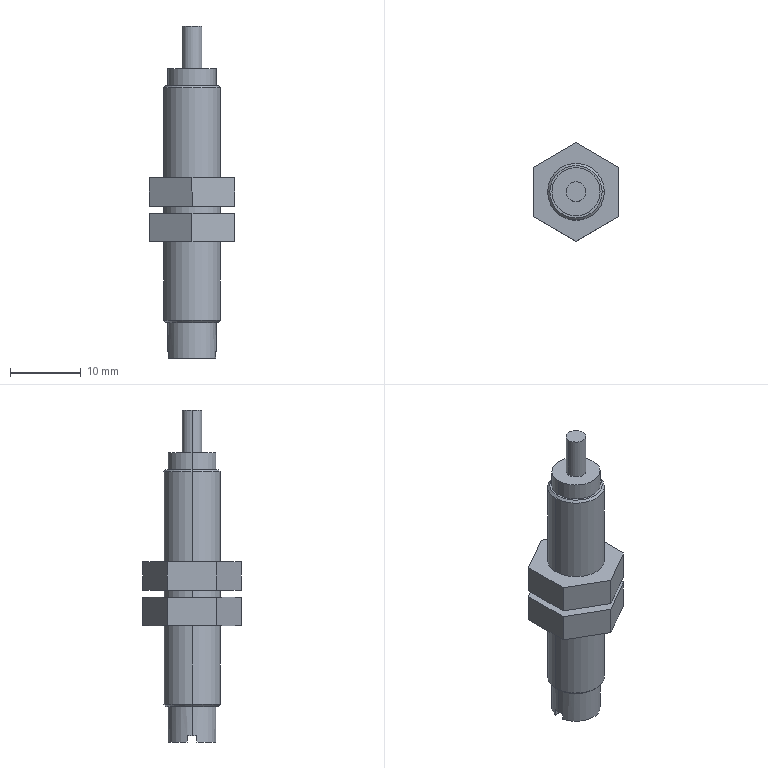Part | SolidWorks | features BaseBody 1 | 1 solid | 41 faces | box 12 x 13.856 x 46.8 mm | volume 2569 mm3 | plane 25 | cylinder 12 | cone 4 | commonest cylinder face diameters 8 x6 6.8 x4 2.8 x2
STEP:
#1=CARTESIAN_POINT('',(1.4,0.,0.));
#2=VERTEX_POINT('',#1);
#3=CARTESIAN_POINT('',(-1.4,0.,0.));
#4=VERTEX_POINT('',#3);
#5=CARTESIAN_POINT('',(0.,0.,0.));
#6=DIRECTION('',(0.,0.,1.));
#7=DIRECTION('',(1.,0.,0.));
#8=AXIS2_PLACEMENT_3D('',#5,#6,#7);
#9=CIRCLE('',#8,1.4);
#10=EDGE_CURVE('',#2,#4,#9,.T.);
#11=ORIENTED_EDGE('',*,*,#10,.T.);
#12=CARTESIAN_POINT('',(-1.4,0.,6.));
#13=VERTEX_POINT('',#12);
#14=CARTESIAN_POINT('',(-1.4,0.,6.));
#15=DIRECTION('',(0.,0.,1.));
#16=VECTOR('',#15,1000.);
#17=LINE('',#14,#16);
#18=EDGE_CURVE('',#4,#13,#17,.T.);
#19=ORIENTED_EDGE('',*,*,#18,.T.);
#20=CARTESIAN_POINT('',(1.4,0.,6.));
#21=VERTEX_POINT('',#20);
#22=CARTESIAN_POINT('',(0.,0.,6.));
#23=DIRECTION('',(0.,0.,-1.));
#24=DIRECTION('',(1.,0.,0.));
#25=AXIS2_PLACEMENT_3D('',#22,#23,#24);
#26=CIRCLE('',#25,1.4);
#27=EDGE_CURVE('',#13,#21,#26,.T.);
#28=ORIENTED_EDGE('',*,*,#27,.T.);
#29=CARTESIAN_POINT('',(1.4,0.,6.));
#30=DIRECTION('',(0.,0.,1.));
#31=VECTOR('',#30,1000.);
#32=LINE('',#29,#31);
#33=EDGE_CURVE('',#2,#21,#32,.T.);
#34=ORIENTED_EDGE('',*,*,#33,.F.);
#35=EDGE_LOOP('',(#11,#19,#28,#34));
#36=FACE_OUTER_BOUND('',#35,.T.);
#37=CARTESIAN_POINT('',(0.,0.,6.));
#38=DIRECTION('',(0.,0.,1.));
#39=DIRECTION('',(1.,0.,0.));
#40=AXIS2_PLACEMENT_3D('',#37,#38,#39);
#41=CYLINDRICAL_SURFACE('',#40,1.4);
#42=ADVANCED_FACE('',(#36),#41,.T.);
#43=CARTESIAN_POINT('',(3.4,0.,-2.4));
#44=VERTEX_POINT('',#43);
#45=CARTESIAN_POINT('',(-3.4,0.,-2.4));
#46=VERTEX_POINT('',#45);
#47=CARTESIAN_POINT('',(0.,0.,-2.4));
#48=DIRECTION('',(0.,0.,1.));
#49=DIRECTION('',(1.,0.,0.));
#50=AXIS2_PLACEMENT_3D('',#47,#48,#49);
#51=CIRCLE('',#50,3.4);
#52=EDGE_CURVE('',#44,#46,#51,.T.);
#53=ORIENTED_EDGE('',*,*,#52,.T.);
#54=CARTESIAN_POINT('',(-3.4,0.,0.));
#55=VERTEX_POINT('',#54);
#56=CARTESIAN_POINT('',(-3.4,0.,0.));
#57=DIRECTION('',(0.,0.,1.));
#58=VECTOR('',#57,1000.);
#59=LINE('',#56,#58);
#60=EDGE_CURVE('',#46,#55,#59,.T.);
#61=ORIENTED_EDGE('',*,*,#60,.T.);
#62=CARTESIAN_POINT('',(3.4,0.,0.));
#63=VERTEX_POINT('',#62);
#64=CARTESIAN_POINT('',(0.,0.,0.));
#65=DIRECTION('',(0.,0.,1.));
#66=DIRECTION('',(1.,0.,0.));
#67=AXIS2_PLACEMENT_3D('',#64,#65,#66);
#68=CIRCLE('',#67,3.4);
#69=EDGE_CURVE('',#63,#55,#68,.T.);
#70=ORIENTED_EDGE('',*,*,#69,.F.);
#71=CARTESIAN_POINT('',(3.4,0.,0.));
#72=DIRECTION('',(0.,0.,1.));
#73=VECTOR('',#72,1000.);
#74=LINE('',#71,#73);
#75=EDGE_CURVE('',#44,#63,#74,.T.);
#76=ORIENTED_EDGE('',*,*,#75,.F.);
#77=EDGE_LOOP('',(#53,#61,#70,#76));
#78=FACE_OUTER_BOUND('',#77,.T.);
#79=CARTESIAN_POINT('',(0.,0.,0.));
#80=DIRECTION('',(0.,0.,1.));
#81=DIRECTION('',(1.,0.,0.));
#82=AXIS2_PLACEMENT_3D('',#79,#80,#81);
#83=CYLINDRICAL_SURFACE('',#82,3.4);
#84=ADVANCED_FACE('',(#78),#83,.T.);
#85=CARTESIAN_POINT('',(3.694,0.,-2.4));
#86=VERTEX_POINT('',#85);
#87=CARTESIAN_POINT('',(-3.694,0.,-2.4));
#88=VERTEX_POINT('',#87);
#89=CARTESIAN_POINT('',(0.,0.,-2.4));
#90=DIRECTION('',(0.,0.,1.));
#91=DIRECTION('',(-1.,0.,0.));
#92=AXIS2_PLACEMENT_3D('',#89,#90,#91);
#93=CIRCLE('',#92,3.694);
#94=EDGE_CURVE('',#86,#88,#93,.T.);
#95=ORIENTED_EDGE('',*,*,#94,.F.);
#96=CARTESIAN_POINT('',(4.,0.,-2.707));
#97=VERTEX_POINT('',#96);
#98=CARTESIAN_POINT('',(3.694,0.,-2.4));
#99=DIRECTION('',(0.7071,0.,-0.7071));
#100=VECTOR('',#99,1000.);
#101=LINE('',#98,#100);
#102=EDGE_CURVE('',#86,#97,#101,.T.);
#103=ORIENTED_EDGE('',*,*,#102,.T.);
#104=CARTESIAN_POINT('',(-4.,0.,-2.707));
#105=VERTEX_POINT('',#104);
#106=CARTESIAN_POINT('',(0.,0.,-2.707));
#107=DIRECTION('',(0.,0.,1.));
#108=DIRECTION('',(0.,1.,0.));
#109=AXIS2_PLACEMENT_3D('',#106,#107,#108);
#110=CIRCLE('',#109,4.);
#111=EDGE_CURVE('',#97,#105,#110,.T.);
#112=ORIENTED_EDGE('',*,*,#111,.T.);
#113=CARTESIAN_POINT('',(-3.694,0.,-2.4));
#114=DIRECTION('',(-0.7071,0.,-0.7071));
#115=VECTOR('',#114,1000.);
#116=LINE('',#113,#115);
#117=EDGE_CURVE('',#88,#105,#116,.T.);
#118=ORIENTED_EDGE('',*,*,#117,.F.);
#119=EDGE_LOOP('',(#95,#103,#112,#118));
#120=FACE_OUTER_BOUND('',#119,.T.);
#121=CARTESIAN_POINT('',(0.,0.,-2.4));
#122=DIRECTION('',(0.,0.,-1.));
#123=DIRECTION('',(-1.,0.,0.));
#124=AXIS2_PLACEMENT_3D('',#121,#122,#123);
#125=CONICAL_SURFACE('',#124,3.694,0.7854);
#126=ADVANCED_FACE('',(#120),#125,.T.);
#127=CARTESIAN_POINT('',(4.,0.,-15.4));
#128=VERTEX_POINT('',#127);
#129=CARTESIAN_POINT('',(-4.,0.,-15.4));
#130=VERTEX_POINT('',#129);
#131=CARTESIAN_POINT('',(0.,0.,-15.4));
#132=DIRECTION('',(0.,0.,1.));
#133=DIRECTION('',(1.,0.,0.));
#134=AXIS2_PLACEMENT_3D('',#131,#132,#133);
#135=CIRCLE('',#134,4.);
#136=EDGE_CURVE('',#128,#130,#135,.T.);
#137=ORIENTED_EDGE('',*,*,#136,.T.);
#138=CARTESIAN_POINT('',(-4.,0.,-2.707));
#139=DIRECTION('',(0.,0.,1.));
#140=VECTOR('',#139,1000.);
#141=LINE('',#138,#140);
#142=EDGE_CURVE('',#130,#105,#141,.T.);
#143=ORIENTED_EDGE('',*,*,#142,.T.);
#144=ORIENTED_EDGE('',*,*,#111,.F.);
#145=CARTESIAN_POINT('',(4.,0.,-2.707));
#146=DIRECTION('',(0.,0.,1.));
#147=VECTOR('',#146,1000.);
#148=LINE('',#145,#147);
#149=EDGE_CURVE('',#128,#97,#148,.T.);
#150=ORIENTED_EDGE('',*,*,#149,.F.);
#151=EDGE_LOOP('',(#137,#143,#144,#150));
#152=FACE_OUTER_BOUND('',#151,.T.);
#153=CARTESIAN_POINT('',(0.,0.,-2.707));
#154=DIRECTION('',(0.,0.,1.));
#155=DIRECTION('',(1.,0.,0.));
#156=AXIS2_PLACEMENT_3D('',#153,#154,#155);
#157=CYLINDRICAL_SURFACE('',#156,4.);
#158=ADVANCED_FACE('',(#152),#157,.T.);
#159=CARTESIAN_POINT('',(4.,0.,-20.4));
#160=VERTEX_POINT('',#159);
#161=CARTESIAN_POINT('',(-4.,0.,-20.4));
#162=VERTEX_POINT('',#161);
#163=CARTESIAN_POINT('',(0.,0.,-20.4));
#164=DIRECTION('',(0.,0.,1.));
#165=DIRECTION('',(1.,0.,0.));
#166=AXIS2_PLACEMENT_3D('',#163,#164,#165);
#167=CIRCLE('',#166,4.);
#168=EDGE_CURVE('',#160,#162,#167,.T.);
#169=ORIENTED_EDGE('',*,*,#168,.T.);
#170=CARTESIAN_POINT('',(-4.,0.,-19.4));
#171=VERTEX_POINT('',#170);
#172=CARTESIAN_POINT('',(-4.,0.,-19.4));
#173=DIRECTION('',(0.,0.,1.));
#174=VECTOR('',#173,1000.);
#175=LINE('',#172,#174);
#176=EDGE_CURVE('',#162,#171,#175,.T.);
#177=ORIENTED_EDGE('',*,*,#176,.T.);
#178=CARTESIAN_POINT('',(4.,0.,-19.4));
#179=VERTEX_POINT('',#178);
#180=CARTESIAN_POINT('',(0.,0.,-19.4));
#181=DIRECTION('',(0.,0.,1.));
#182=DIRECTION('',(1.,0.,0.));
#183=AXIS2_PLACEMENT_3D('',#180,#181,#182);
#184=CIRCLE('',#183,4.);
#185=EDGE_CURVE('',#179,#171,#184,.T.);
#186=ORIENTED_EDGE('',*,*,#185,.F.);
#187=CARTESIAN_POINT('',(4.,0.,-19.4));
#188=DIRECTION('',(0.,0.,1.));
#189=VECTOR('',#188,1000.);
#190=LINE('',#187,#189);
#191=EDGE_CURVE('',#160,#179,#190,.T.);
#192=ORIENTED_EDGE('',*,*,#191,.F.);
#193=EDGE_LOOP('',(#169,#177,#186,#192));
#194=FACE_OUTER_BOUND('',#193,.T.);
#195=CARTESIAN_POINT('',(0.,0.,-19.4));
#196=DIRECTION('',(0.,0.,1.));
#197=DIRECTION('',(1.,0.,0.));
#198=AXIS2_PLACEMENT_3D('',#195,#196,#197);
#199=CYLINDRICAL_SURFACE('',#198,4.);
#200=ADVANCED_FACE('',(#194),#199,.T.);
#201=CARTESIAN_POINT('',(4.,0.,-35.494));
#202=VERTEX_POINT('',#201);
#203=CARTESIAN_POINT('',(-4.,0.,-35.494));
#204=VERTEX_POINT('',#203);
#205=CARTESIAN_POINT('',(0.,0.,-35.494));
#206=DIRECTION('',(0.,0.,1.));
#207=DIRECTION('',(0.,1.,0.));
#208=AXIS2_PLACEMENT_3D('',#205,#206,#207);
#209=CIRCLE('',#208,4.);
#210=EDGE_CURVE('',#202,#204,#209,.T.);
#211=ORIENTED_EDGE('',*,*,#210,.T.);
#212=CARTESIAN_POINT('',(-4.,0.,-24.4));
#213=VERTEX_POINT('',#212);
#214=CARTESIAN_POINT('',(-4.,0.,-24.4));
#215=DIRECTION('',(0.,0.,1.));
#216=VECTOR('',#215,1000.);
#217=LINE('',#214,#216);
#218=EDGE_CURVE('',#204,#213,#217,.T.);
#219=ORIENTED_EDGE('',*,*,#218,.T.);
#220=CARTESIAN_POINT('',(4.,0.,-24.4));
#221=VERTEX_POINT('',#220);
#222=CARTESIAN_POINT('',(0.,0.,-24.4));
#223=DIRECTION('',(0.,0.,1.));
#224=DIRECTION('',(1.,0.,0.));
#225=AXIS2_PLACEMENT_3D('',#222,#223,#224);
#226=CIRCLE('',#225,4.);
#227=EDGE_CURVE('',#221,#213,#226,.T.);
#228=ORIENTED_EDGE('',*,*,#227,.F.);
#229=CARTESIAN_POINT('',(4.,0.,-24.4));
#230=DIRECTION('',(0.,0.,1.));
#231=VECTOR('',#230,1000.);
#232=LINE('',#229,#231);
#233=EDGE_CURVE('',#202,#221,#232,.T.);
#234=ORIENTED_EDGE('',*,*,#233,.F.);
#235=EDGE_LOOP('',(#211,#219,#228,#234));
#236=FACE_OUTER_BOUND('',#235,.T.);
#237=CARTESIAN_POINT('',(0.,0.,-24.4));
#238=DIRECTION('',(0.,0.,1.));
#239=DIRECTION('',(1.,0.,0.));
#240=AXIS2_PLACEMENT_3D('',#237,#238,#239);
#241=CYLINDRICAL_SURFACE('',#240,4.);
#242=ADVANCED_FACE('',(#236),#241,.T.);
#243=CARTESIAN_POINT('',(3.693,0.,-35.8));
#244=VERTEX_POINT('',#243);
#245=CARTESIAN_POINT('',(-3.693,0.,-35.8));
#246=VERTEX_POINT('',#245);
#247=CARTESIAN_POINT('',(0.,0.,-35.8));
#248=DIRECTION('',(0.,0.,1.));
#249=DIRECTION('',(1.,0.,0.));
#250=AXIS2_PLACEMENT_3D('',#247,#248,#249);
#251=CIRCLE('',#250,3.693);
#252=EDGE_CURVE('',#244,#246,#251,.T.);
#253=ORIENTED_EDGE('',*,*,#252,.T.);
#254=CARTESIAN_POINT('',(-3.693,0.,-35.8));
#255=DIRECTION('',(-0.7071,0.,0.7071));
#256=VECTOR('',#255,1000.);
#257=LINE('',#254,#256);
#258=EDGE_CURVE('',#246,#204,#257,.T.);
#259=ORIENTED_EDGE('',*,*,#258,.T.);
#260=ORIENTED_EDGE('',*,*,#210,.F.);
#261=CARTESIAN_POINT('',(3.693,0.,-35.8));
#262=DIRECTION('',(0.7071,0.,0.7071));
#263=VECTOR('',#262,1000.);
#264=LINE('',#261,#263);
#265=EDGE_CURVE('',#244,#202,#264,.T.);
#266=ORIENTED_EDGE('',*,*,#265,.F.);
#267=EDGE_LOOP('',(#253,#259,#260,#266));
#268=FACE_OUTER_BOUND('',#267,.T.);
#269=CARTESIAN_POINT('',(0.,0.,-35.8));
#270=DIRECTION('',(0.,0.,1.));
#271=DIRECTION('',(1.,0.,0.));
#272=AXIS2_PLACEMENT_3D('',#269,#270,#271);
#273=CONICAL_SURFACE('',#272,3.693,0.7854);
#274=ADVANCED_FACE('',(#268),#273,.T.);
#275=CARTESIAN_POINT('',(-3.4,0.,-39.9));
#276=VERTEX_POINT('',#275);
#277=CARTESIAN_POINT('',(-3.327,0.7,-39.9));
#278=VERTEX_POINT('',#277);
#279=CARTESIAN_POINT('',(0.,0.,-39.9));
#280=DIRECTION('',(0.,0.,-1.));
#281=DIRECTION('',(1.,0.,0.));
#282=AXIS2_PLACEMENT_3D('',#279,#280,#281);
#283=CIRCLE('',#282,3.4);
#284=EDGE_CURVE('',#276,#278,#283,.T.);
#285=ORIENTED_EDGE('',*,*,#284,.F.);
#286=CARTESIAN_POINT('',(-3.4,0.,-35.8));
#287=VERTEX_POINT('',#286);
#288=CARTESIAN_POINT('',(-3.4,0.,-35.8));
#289=DIRECTION('',(0.,0.,1.));
#290=VECTOR('',#289,1000.);
#291=LINE('',#288,#290);
#292=EDGE_CURVE('',#276,#287,#291,.T.);
#293=ORIENTED_EDGE('',*,*,#292,.T.);
#294=CARTESIAN_POINT('',(3.4,0.,-35.8));
#295=VERTEX_POINT('',#294);
#296=CARTESIAN_POINT('',(0.,0.,-35.8));
#297=DIRECTION('',(0.,0.,1.));
#298=DIRECTION('',(1.,0.,0.));
#299=AXIS2_PLACEMENT_3D('',#296,#297,#298);
#300=CIRCLE('',#299,3.4);
#301=EDGE_CURVE('',#295,#287,#300,.T.);
#302=ORIENTED_EDGE('',*,*,#301,.F.);
#303=CARTESIAN_POINT('',(3.4,0.,-39.9));
#304=VERTEX_POINT('',#303);
#305=CARTESIAN_POINT('',(3.4,0.,-35.8));
#306=DIRECTION('',(0.,0.,1.));
#307=VECTOR('',#306,1000.);
#308=LINE('',#305,#307);
#309=EDGE_CURVE('',#304,#295,#308,.T.);
#310=ORIENTED_EDGE('',*,*,#309,.F.);
#311=CARTESIAN_POINT('',(3.327,0.7,-39.9));
#312=VERTEX_POINT('',#311);
#313=CARTESIAN_POINT('',(0.,0.,-39.9));
#314=DIRECTION('',(0.,0.,-1.));
#315=DIRECTION('',(1.,0.,0.));
#316=AXIS2_PLACEMENT_3D('',#313,#314,#315);
#317=CIRCLE('',#316,3.4);
#318=EDGE_CURVE('',#312,#304,#317,.T.);
#319=ORIENTED_EDGE('',*,*,#318,.F.);
#320=CARTESIAN_POINT('',(3.327,0.7,-40.8));
#321=VERTEX_POINT('',#320);
#322=CARTESIAN_POINT('',(3.327,0.7,-40.35));
#323=DIRECTION('',(0.,0.,1.));
#324=VECTOR('',#323,1000.);
#325=LINE('',#322,#324);
#326=EDGE_CURVE('',#321,#312,#325,.T.);
#327=ORIENTED_EDGE('',*,*,#326,.F.);
#328=CARTESIAN_POINT('',(-3.327,0.7,-40.8));
#329=VERTEX_POINT('',#328);
#330=CARTESIAN_POINT('',(0.,0.,-40.8));
#331=DIRECTION('',(0.,0.,1.));
#332=DIRECTION('',(1.,0.,0.));
#333=AXIS2_PLACEMENT_3D('',#330,#331,#332);
#334=CIRCLE('',#333,3.4);
#335=EDGE_CURVE('',#321,#329,#334,.T.);
#336=ORIENTED_EDGE('',*,*,#335,.T.);
#337=CARTESIAN_POINT('',(-3.327,0.7,-40.35));
#338=DIRECTION('',(0.,0.,-1.));
#339=VECTOR('',#338,1000.);
#340=LINE('',#337,#339);
#341=EDGE_CURVE('',#278,#329,#340,.T.);
#342=ORIENTED_EDGE('',*,*,#341,.F.);
#343=EDGE_LOOP('',(#285,#293,#302,#310,#319,#327,#336,#342));
#344=FACE_OUTER_BOUND('',#343,.T.);
#345=CARTESIAN_POINT('',(0.,0.,-35.8));
#346=DIRECTION('',(0.,0.,1.));
#347=DIRECTION('',(1.,0.,0.));
#348=AXIS2_PLACEMENT_3D('',#345,#346,#347);
#349=CYLINDRICAL_SURFACE('',#348,3.4);
#350=ADVANCED_FACE('',(#344),#349,.T.);
#351=ORIENTED_EDGE('',*,*,#18,.F.);
#352=CARTESIAN_POINT('',(0.,0.,0.));
#353=DIRECTION('',(0.,0.,1.));
#354=DIRECTION('',(1.,0.,0.));
#355=AXIS2_PLACEMENT_3D('',#352,#353,#354);
#356=CIRCLE('',#355,1.4);
#357=EDGE_CURVE('',#4,#2,#356,.T.);
#358=ORIENTED_EDGE('',*,*,#357,.T.);
#359=ORIENTED_EDGE('',*,*,#33,.T.);
#360=CARTESIAN_POINT('',(0.,0.,6.));
#361=DIRECTION('',(0.,0.,-1.));
#362=DIRECTION('',(1.,0.,0.));
#363=AXIS2_PLACEMENT_3D('',#360,#361,#362);
#364=CIRCLE('',#363,1.4);
#365=EDGE_CURVE('',#21,#13,#364,.T.);
#366=ORIENTED_EDGE('',*,*,#365,.T.);
#367=EDGE_LOOP('',(#351,#358,#359,#366));
#368=FACE_OUTER_BOUND('',#367,.T.);
#369=CARTESIAN_POINT('',(0.,0.,6.));
#370=DIRECTION('',(0.,0.,1.));
#371=DIRECTION('',(1.,0.,0.));
#372=AXIS2_PLACEMENT_3D('',#369,#370,#371);
#373=CYLINDRICAL_SURFACE('',#372,1.4);
#374=ADVANCED_FACE('',(#368),#373,.T.);
#375=ORIENTED_EDGE('',*,*,#365,.F.);
#376=ORIENTED_EDGE('',*,*,#27,.F.);
#377=EDGE_LOOP('',(#375,#376));
#378=FACE_OUTER_BOUND('',#377,.T.);
#379=CARTESIAN_POINT('',(1.417,-1.4,6.));
#380=DIRECTION('',(0.,0.,1.));
#381=DIRECTION('',(0.,1.,0.));
#382=AXIS2_PLACEMENT_3D('',#379,#380,#381);
#383=PLANE('',#382);
#384=ADVANCED_FACE('',(#378),#383,.T.);
#385=ORIENTED_EDGE('',*,*,#10,.F.);
#386=ORIENTED_EDGE('',*,*,#357,.F.);
#387=EDGE_LOOP('',(#385,#386));
#388=FACE_BOUND('',#387,.T.);
#389=ORIENTED_EDGE('',*,*,#69,.T.);
#390=CARTESIAN_POINT('',(0.,0.,0.));
#391=DIRECTION('',(0.,0.,1.));
#392=DIRECTION('',(1.,0.,0.));
#393=AXIS2_PLACEMENT_3D('',#390,#391,#392);
#394=CIRCLE('',#393,3.4);
#395=EDGE_CURVE('',#55,#63,#394,.T.);
#396=ORIENTED_EDGE('',*,*,#395,.T.);
#397=EDGE_LOOP('',(#389,#396));
#398=FACE_OUTER_BOUND('',#397,.T.);
#399=CARTESIAN_POINT('',(3.441,-3.4,0.));
#400=DIRECTION('',(0.,0.,1.));
#401=DIRECTION('',(0.,1.,0.));
#402=AXIS2_PLACEMENT_3D('',#399,#400,#401);
#403=PLANE('',#402);
#404=ADVANCED_FACE('',(#388,#398),#403,.T.);
#405=ORIENTED_EDGE('',*,*,#60,.F.);
#406=CARTESIAN_POINT('',(0.,0.,-2.4));
#407=DIRECTION('',(0.,0.,1.));
#408=DIRECTION('',(1.,0.,0.));
#409=AXIS2_PLACEMENT_3D('',#406,#407,#408);
#410=CIRCLE('',#409,3.4);
#411=EDGE_CURVE('',#46,#44,#410,.T.);
#412=ORIENTED_EDGE('',*,*,#411,.T.);
#413=ORIENTED_EDGE('',*,*,#75,.T.);
#414=ORIENTED_EDGE('',*,*,#395,.F.);
#415=EDGE_LOOP('',(#405,#412,#413,#414));
#416=FACE_OUTER_BOUND('',#415,.T.);
#417=CARTESIAN_POINT('',(0.,0.,0.));
#418=DIRECTION('',(0.,0.,1.));
#419=DIRECTION('',(1.,0.,0.));
#420=AXIS2_PLACEMENT_3D('',#417,#418,#419);
#421=CYLINDRICAL_SURFACE('',#420,3.4);
#422=ADVANCED_FACE('',(#416),#421,.T.);
#423=ORIENTED_EDGE('',*,*,#52,.F.);
#424=ORIENTED_EDGE('',*,*,#411,.F.);
#425=EDGE_LOOP('',(#423,#424));
#426=FACE_BOUND('',#425,.T.);
#427=CARTESIAN_POINT('',(0.,0.,-2.4));
#428=DIRECTION('',(0.,0.,1.));
#429=DIRECTION('',(-1.,0.,0.));
#430=AXIS2_PLACEMENT_3D('',#427,#428,#429);
#431=CIRCLE('',#430,3.694);
#432=EDGE_CURVE('',#88,#86,#431,.T.);
#433=ORIENTED_EDGE('',*,*,#432,.T.);
#434=ORIENTED_EDGE('',*,*,#94,.T.);
#435=EDGE_LOOP('',(#433,#434));
#436=FACE_OUTER_BOUND('',#435,.T.);
#437=CARTESIAN_POINT('',(3.738,-3.694,-2.4));
#438=DIRECTION('',(0.,0.,1.));
#439=DIRECTION('',(0.,1.,0.));
#440=AXIS2_PLACEMENT_3D('',#437,#438,#439);
#441=PLANE('',#440);
#442=ADVANCED_FACE('',(#426,#436),#441,.T.);
#443=ORIENTED_EDGE('',*,*,#102,.F.);
#444=ORIENTED_EDGE('',*,*,#432,.F.);
#445=ORIENTED_EDGE('',*,*,#117,.T.);
#446=CARTESIAN_POINT('',(0.,0.,-2.707));
#447=DIRECTION('',(0.,0.,1.));
#448=DIRECTION('',(0.,1.,0.));
#449=AXIS2_PLACEMENT_3D('',#446,#447,#448);
#450=CIRCLE('',#449,4.);
#451=EDGE_CURVE('',#105,#97,#450,.T.);
#452=ORIENTED_EDGE('',*,*,#451,.T.);
#453=EDGE_LOOP('',(#443,#444,#445,#452));
#454=FACE_OUTER_BOUND('',#453,.T.);
#455=CARTESIAN_POINT('',(0.,0.,-2.4));
#456=DIRECTION('',(0.,0.,-1.));
#457=DIRECTION('',(-1.,0.,0.));
#458=AXIS2_PLACEMENT_3D('',#455,#456,#457);
#459=CONICAL_SURFACE('',#458,3.694,0.7854);
#460=ADVANCED_FACE('',(#454),#459,.T.);
#461=ORIENTED_EDGE('',*,*,#142,.F.);
#462=CARTESIAN_POINT('',(0.,0.,-15.4));
#463=DIRECTION('',(0.,0.,1.));
#464=DIRECTION('',(1.,0.,0.));
#465=AXIS2_PLACEMENT_3D('',#462,#463,#464);
#466=CIRCLE('',#465,4.);
#467=EDGE_CURVE('',#130,#128,#466,.T.);
#468=ORIENTED_EDGE('',*,*,#467,.T.);
#469=ORIENTED_EDGE('',*,*,#149,.T.);
#470=ORIENTED_EDGE('',*,*,#451,.F.);
#471=EDGE_LOOP('',(#461,#468,#469,#470));
#472=FACE_OUTER_BOUND('',#471,.T.);
#473=CARTESIAN_POINT('',(0.,0.,-2.707));
#474=DIRECTION('',(0.,0.,1.));
#475=DIRECTION('',(1.,0.,0.));
#476=AXIS2_PLACEMENT_3D('',#473,#474,#475);
#477=CYLINDRICAL_SURFACE('',#476,4.);
#478=ADVANCED_FACE('',(#472),#477,.T.);
#479=ORIENTED_EDGE('',*,*,#136,.F.);
#480=ORIENTED_EDGE('',*,*,#467,.F.);
#481=EDGE_LOOP('',(#479,#480));
#482=FACE_BOUND('',#481,.T.);
#483=CARTESIAN_POINT('',(6.,-3.464,-15.4));
#484=VERTEX_POINT('',#483);
#485=CARTESIAN_POINT('',(6.,3.464,-15.4));
#486=VERTEX_POINT('',#485);
#487=CARTESIAN_POINT('',(6.,-6.928,-15.4));
#488=DIRECTION('',(0.,1.,0.));
#489=VECTOR('',#488,1000.);
#490=LINE('',#487,#489);
#491=EDGE_CURVE('',#484,#486,#490,.T.);
#492=ORIENTED_EDGE('',*,*,#491,.T.);
#493=CARTESIAN_POINT('',(-0.000000108,6.928,-15.4));
#494=VERTEX_POINT('',#493);
#495=CARTESIAN_POINT('',(6.,3.464,-15.4));
#496=CARTESIAN_POINT('',(4.,4.619,-15.4));
#497=CARTESIAN_POINT('',(2.,5.774,-15.4));
#498=CARTESIAN_POINT('',(-0.000000108,6.928,-15.4));
#499=B_SPLINE_CURVE_WITH_KNOTS('',3,(#495,#496,#497,#498),.UNSPECIFIED.,.F.,.F.,(4,4),(0.,1.),.UNSPECIFIED.);
#500=EDGE_CURVE('',#486,#494,#499,.T.);
#501=ORIENTED_EDGE('',*,*,#500,.T.);
#502=CARTESIAN_POINT('',(-6.,3.464,-15.4));
#503=VERTEX_POINT('',#502);
#504=CARTESIAN_POINT('',(-0.000000108,6.928,-15.4));
#505=CARTESIAN_POINT('',(-2.,5.774,-15.4));
#506=CARTESIAN_POINT('',(-4.,4.619,-15.4));
#507=CARTESIAN_POINT('',(-6.,3.464,-15.4));
#508=B_SPLINE_CURVE_WITH_KNOTS('',3,(#504,#505,#506,#507),.UNSPECIFIED.,.F.,.F.,(4,4),(0.000000018,1.),.UNSPECIFIED.);
#509=EDGE_CURVE('',#494,#503,#508,.T.);
#510=ORIENTED_EDGE('',*,*,#509,.T.);
#511=CARTESIAN_POINT('',(-6.,-3.464,-15.4));
#512=VERTEX_POINT('',#511);
#513=CARTESIAN_POINT('',(-6.,-6.928,-15.4));
#514=DIRECTION('',(0.,-1.,0.));
#515=VECTOR('',#514,1000.);
#516=LINE('',#513,#515);
#517=EDGE_CURVE('',#503,#512,#516,.T.);
#518=ORIENTED_EDGE('',*,*,#517,.T.);
#519=CARTESIAN_POINT('',(-0.000000108,-6.928,-15.4));
#520=VERTEX_POINT('',#519);
#521=CARTESIAN_POINT('',(-6.,-3.464,-15.4));
#522=CARTESIAN_POINT('',(-4.,-4.619,-15.4));
#523=CARTESIAN_POINT('',(-2.,-5.774,-15.4));
#524=CARTESIAN_POINT('',(-0.000000108,-6.928,-15.4));
#525=B_SPLINE_CURVE_WITH_KNOTS('',3,(#521,#522,#523,#524),.UNSPECIFIED.,.F.,.F.,(4,4),(0.,1.),.UNSPECIFIED.);
#526=EDGE_CURVE('',#512,#520,#525,.T.);
#527=ORIENTED_EDGE('',*,*,#526,.T.);
#528=CARTESIAN_POINT('',(-0.000000108,-6.928,-15.4));
#529=CARTESIAN_POINT('',(2.,-5.774,-15.4));
#530=CARTESIAN_POINT('',(4.,-4.619,-15.4));
#531=CARTESIAN_POINT('',(6.,-3.464,-15.4));
#532=B_SPLINE_CURVE_WITH_KNOTS('',3,(#528,#529,#530,#531),.UNSPECIFIED.,.F.,.F.,(4,4),(0.,1.),.UNSPECIFIED.);
#533=EDGE_CURVE('',#520,#484,#532,.T.);
#534=ORIENTED_EDGE('',*,*,#533,.T.);
#535=EDGE_LOOP('',(#492,#501,#510,#518,#527,#534));
#536=FACE_OUTER_BOUND('',#535,.T.);
#537=CARTESIAN_POINT('',(-6.,-7.011,-15.4));
#538=DIRECTION('',(0.,0.,1.));
#539=DIRECTION('',(1.,0.,0.));
#540=AXIS2_PLACEMENT_3D('',#537,#538,#539);
#541=PLANE('',#540);
#542=ADVANCED_FACE('',(#482,#536),#541,.T.);
#543=CARTESIAN_POINT('',(6.,3.464,-19.4));
#544=VERTEX_POINT('',#543);
#545=CARTESIAN_POINT('',(-0.000000217,6.928,-19.4));
#546=VERTEX_POINT('',#545);
#547=CARTESIAN_POINT('',(3.,5.196,-19.4));
#548=DIRECTION('',(-0.866,0.5,0.));
#549=VECTOR('',#548,1000.);
#550=LINE('',#547,#549);
#551=EDGE_CURVE('',#544,#546,#550,.T.);
#552=ORIENTED_EDGE('',*,*,#551,.T.);
#553=CARTESIAN_POINT('',(0.,6.928,-19.4));
#554=DIRECTION('',(0.,0.,1.));
#555=VECTOR('',#554,1000.);
#556=LINE('',#553,#555);
#557=EDGE_CURVE('',#546,#494,#556,.T.);
#558=ORIENTED_EDGE('',*,*,#557,.T.);
#559=ORIENTED_EDGE('',*,*,#500,.F.);
#560=CARTESIAN_POINT('',(6.,3.464,-19.4));
#561=DIRECTION('',(0.,0.,-1.));
#562=VECTOR('',#561,1000.);
#563=LINE('',#560,#562);
#564=EDGE_CURVE('',#486,#544,#563,.T.);
#565=ORIENTED_EDGE('',*,*,#564,.T.);
#566=EDGE_LOOP('',(#552,#558,#559,#565));
#567=FACE_OUTER_BOUND('',#566,.T.);
#568=CARTESIAN_POINT('',(6.,3.464,-19.4));
#569=DIRECTION('',(0.5,0.866,0.));
#570=DIRECTION('',(-0.866,0.5,0.));
#571=AXIS2_PLACEMENT_3D('',#568,#569,#570);
#572=PLANE('',#571);
#573=ADVANCED_FACE('',(#567),#572,.T.);
#574=CARTESIAN_POINT('',(6.,-3.464,-19.4));
#575=VERTEX_POINT('',#574);
#576=CARTESIAN_POINT('',(6.,0.,-19.4));
#577=DIRECTION('',(0.,1.,0.));
#578=VECTOR('',#577,1000.);
#579=LINE('',#576,#578);
#580=EDGE_CURVE('',#575,#544,#579,.T.);
#581=ORIENTED_EDGE('',*,*,#580,.T.);
#582=ORIENTED_EDGE('',*,*,#564,.F.);
#583=ORIENTED_EDGE('',*,*,#491,.F.);
#584=CARTESIAN_POINT('',(6.,-3.464,-19.4));
#585=DIRECTION('',(0.,0.,-1.));
#586=VECTOR('',#585,1000.);
#587=LINE('',#584,#586);
#588=EDGE_CURVE('',#484,#575,#587,.T.);
#589=ORIENTED_EDGE('',*,*,#588,.T.);
#590=EDGE_LOOP('',(#581,#582,#583,#589));
#591=FACE_OUTER_BOUND('',#590,.T.);
#592=CARTESIAN_POINT('',(6.,-3.464,-19.4));
#593=DIRECTION('',(1.,0.,0.));
#594=DIRECTION('',(0.,1.,0.));
#595=AXIS2_PLACEMENT_3D('',#592,#593,#594);
#596=PLANE('',#595);
#597=ADVANCED_FACE('',(#591),#596,.T.);
#598=CARTESIAN_POINT('',(0.000000108,-6.928,-19.4));
#599=VERTEX_POINT('',#598);
#600=CARTESIAN_POINT('',(3.,-5.196,-19.4));
#601=DIRECTION('',(0.866,0.5,0.));
#602=VECTOR('',#601,1000.);
#603=LINE('',#600,#602);
#604=EDGE_CURVE('',#599,#575,#603,.T.);
#605=ORIENTED_EDGE('',*,*,#604,.T.);
#606=ORIENTED_EDGE('',*,*,#588,.F.);
#607=ORIENTED_EDGE('',*,*,#533,.F.);
#608=CARTESIAN_POINT('',(0.,-6.928,-19.4));
#609=DIRECTION('',(0.,0.,-1.));
#610=VECTOR('',#609,1000.);
#611=LINE('',#608,#610);
#612=EDGE_CURVE('',#520,#599,#611,.T.);
#613=ORIENTED_EDGE('',*,*,#612,.T.);
#614=EDGE_LOOP('',(#605,#606,#607,#613));
#615=FACE_OUTER_BOUND('',#614,.T.);
#616=CARTESIAN_POINT('',(0.,-6.928,-19.4));
#617=DIRECTION('',(0.5,-0.866,0.));
#618=DIRECTION('',(0.866,0.5,0.));
#619=AXIS2_PLACEMENT_3D('',#616,#617,#618);
#620=PLANE('',#619);
#621=ADVANCED_FACE('',(#615),#620,.T.);
#622=CARTESIAN_POINT('',(-6.,-3.464,-19.4));
#623=VERTEX_POINT('',#622);
#624=CARTESIAN_POINT('',(-3.,-5.196,-19.4));
#625=DIRECTION('',(0.866,-0.5,0.));
#626=VECTOR('',#625,1000.);
#627=LINE('',#624,#626);
#628=EDGE_CURVE('',#623,#599,#627,.T.);
#629=ORIENTED_EDGE('',*,*,#628,.T.);
#630=ORIENTED_EDGE('',*,*,#612,.F.);
#631=ORIENTED_EDGE('',*,*,#526,.F.);
#632=CARTESIAN_POINT('',(-6.,-3.464,-19.4));
#633=DIRECTION('',(0.,0.,-1.));
#634=VECTOR('',#633,1000.);
#635=LINE('',#632,#634);
#636=EDGE_CURVE('',#512,#623,#635,.T.);
#637=ORIENTED_EDGE('',*,*,#636,.T.);
#638=EDGE_LOOP('',(#629,#630,#631,#637));
#639=FACE_OUTER_BOUND('',#638,.T.);
#640=CARTESIAN_POINT('',(-6.,-3.464,-19.4));
#641=DIRECTION('',(-0.5,-0.866,0.));
#642=DIRECTION('',(0.866,-0.5,0.));
#643=AXIS2_PLACEMENT_3D('',#640,#641,#642);
#644=PLANE('',#643);
#645=ADVANCED_FACE('',(#639),#644,.T.);
#646=CARTESIAN_POINT('',(-6.,3.464,-19.4));
#647=VERTEX_POINT('',#646);
#648=CARTESIAN_POINT('',(-6.,0.,-19.4));
#649=DIRECTION('',(0.,-1.,0.));
#650=VECTOR('',#649,1000.);
#651=LINE('',#648,#650);
#652=EDGE_CURVE('',#647,#623,#651,.T.);
#653=ORIENTED_EDGE('',*,*,#652,.T.);
#654=ORIENTED_EDGE('',*,*,#636,.F.);
#655=ORIENTED_EDGE('',*,*,#517,.F.);
#656=CARTESIAN_POINT('',(-6.,3.464,-19.4));
#657=DIRECTION('',(0.,0.,-1.));
#658=VECTOR('',#657,1000.);
#659=LINE('',#656,#658);
#660=EDGE_CURVE('',#503,#647,#659,.T.);
#661=ORIENTED_EDGE('',*,*,#660,.T.);
#662=EDGE_LOOP('',(#653,#654,#655,#661));
#663=FACE_OUTER_BOUND('',#662,.T.);
#664=CARTESIAN_POINT('',(-6.,3.464,-19.4));
#665=DIRECTION('',(-1.,0.,0.));
#666=DIRECTION('',(0.,-1.,0.));
#667=AXIS2_PLACEMENT_3D('',#664,#665,#666);
#668=PLANE('',#667);
#669=ADVANCED_FACE('',(#663),#668,.T.);
#670=CARTESIAN_POINT('',(-3.,5.196,-19.4));
#671=DIRECTION('',(-0.866,-0.5,0.));
#672=VECTOR('',#671,1000.);
#673=LINE('',#670,#672);
#674=EDGE_CURVE('',#546,#647,#673,.T.);
#675=ORIENTED_EDGE('',*,*,#674,.T.);
#676=ORIENTED_EDGE('',*,*,#660,.F.);
#677=ORIENTED_EDGE('',*,*,#509,.F.);
#678=ORIENTED_EDGE('',*,*,#557,.F.);
#679=EDGE_LOOP('',(#675,#676,#677,#678));
#680=FACE_OUTER_BOUND('',#679,.T.);
#681=CARTESIAN_POINT('',(0.,6.928,-19.4));
#682=DIRECTION('',(-0.5,0.866,0.));
#683=DIRECTION('',(-0.866,-0.5,0.));
#684=AXIS2_PLACEMENT_3D('',#681,#682,#683);
#685=PLANE('',#684);
#686=ADVANCED_FACE('',(#680),#685,.T.);
#687=ORIENTED_EDGE('',*,*,#185,.T.);
#688=CARTESIAN_POINT('',(0.,0.,-19.4));
#689=DIRECTION('',(0.,0.,1.));
#690=DIRECTION('',(1.,0.,0.));
#691=AXIS2_PLACEMENT_3D('',#688,#689,#690);
#692=CIRCLE('',#691,4.);
#693=EDGE_CURVE('',#171,#179,#692,.T.);
#694=ORIENTED_EDGE('',*,*,#693,.T.);
#695=EDGE_LOOP('',(#687,#694));
#696=FACE_BOUND('',#695,.T.);
#697=ORIENTED_EDGE('',*,*,#604,.F.);
#698=ORIENTED_EDGE('',*,*,#628,.F.);
#699=ORIENTED_EDGE('',*,*,#652,.F.);
#700=ORIENTED_EDGE('',*,*,#674,.F.);
#701=ORIENTED_EDGE('',*,*,#551,.F.);
#702=ORIENTED_EDGE('',*,*,#580,.F.);
#703=EDGE_LOOP('',(#697,#698,#699,#700,#701,#702));
#704=FACE_OUTER_BOUND('',#703,.T.);
#705=CARTESIAN_POINT('',(6.,-7.011,-19.4));
#706=DIRECTION('',(0.,0.,-1.));
#707=DIRECTION('',(-1.,0.,0.));
#708=AXIS2_PLACEMENT_3D('',#705,#706,#707);
#709=PLANE('',#708);
#710=ADVANCED_FACE('',(#696,#704),#709,.T.);
#711=ORIENTED_EDGE('',*,*,#176,.F.);
#712=CARTESIAN_POINT('',(0.,0.,-20.4));
#713=DIRECTION('',(0.,0.,1.));
#714=DIRECTION('',(1.,0.,0.));
#715=AXIS2_PLACEMENT_3D('',#712,#713,#714);
#716=CIRCLE('',#715,4.);
#717=EDGE_CURVE('',#162,#160,#716,.T.);
#718=ORIENTED_EDGE('',*,*,#717,.T.);
#719=ORIENTED_EDGE('',*,*,#191,.T.);
#720=ORIENTED_EDGE('',*,*,#693,.F.);
#721=EDGE_LOOP('',(#711,#718,#719,#720));
#722=FACE_OUTER_BOUND('',#721,.T.);
#723=CARTESIAN_POINT('',(0.,0.,-19.4));
#724=DIRECTION('',(0.,0.,1.));
#725=DIRECTION('',(1.,0.,0.));
#726=AXIS2_PLACEMENT_3D('',#723,#724,#725);
#727=CYLINDRICAL_SURFACE('',#726,4.);
#728=ADVANCED_FACE('',(#722),#727,.T.);
#729=ORIENTED_EDGE('',*,*,#168,.F.);
#730=ORIENTED_EDGE('',*,*,#717,.F.);
#731=EDGE_LOOP('',(#729,#730));
#732=FACE_BOUND('',#731,.T.);
#733=CARTESIAN_POINT('',(6.,3.464,-20.4));
#734=VERTEX_POINT('',#733);
#735=CARTESIAN_POINT('',(0.000000108,6.928,-20.4));
#736=VERTEX_POINT('',#735);
#737=CARTESIAN_POINT('',(6.,3.464,-20.4));
#738=CARTESIAN_POINT('',(4.,4.619,-20.4));
#739=CARTESIAN_POINT('',(2.,5.774,-20.4));
#740=CARTESIAN_POINT('',(0.000000108,6.928,-20.4));
#741=B_SPLINE_CURVE_WITH_KNOTS('',3,(#737,#738,#739,#740),.UNSPECIFIED.,.F.,.F.,(4,4),(0.,1.),.UNSPECIFIED.);
#742=EDGE_CURVE('',#734,#736,#741,.T.);
#743=ORIENTED_EDGE('',*,*,#742,.T.);
#744=CARTESIAN_POINT('',(-6.,3.464,-20.4));
#745=VERTEX_POINT('',#744);
#746=CARTESIAN_POINT('',(0.000000108,6.928,-20.4));
#747=CARTESIAN_POINT('',(-2.,5.774,-20.4));
#748=CARTESIAN_POINT('',(-4.,4.619,-20.4));
#749=CARTESIAN_POINT('',(-6.,3.464,-20.4));
#750=B_SPLINE_CURVE_WITH_KNOTS('',3,(#746,#747,#748,#749),.UNSPECIFIED.,.F.,.F.,(4,4),(0.,1.),.UNSPECIFIED.);
#751=EDGE_CURVE('',#736,#745,#750,.T.);
#752=ORIENTED_EDGE('',*,*,#751,.T.);
#753=CARTESIAN_POINT('',(-6.,-3.464,-20.4));
#754=VERTEX_POINT('',#753);
#755=CARTESIAN_POINT('',(-6.,-6.928,-20.4));
#756=DIRECTION('',(0.,-1.,0.));
#757=VECTOR('',#756,1000.);
#758=LINE('',#755,#757);
#759=EDGE_CURVE('',#745,#754,#758,.T.);
#760=ORIENTED_EDGE('',*,*,#759,.T.);
#761=CARTESIAN_POINT('',(-0.000000108,-6.928,-20.4));
#762=VERTEX_POINT('',#761);
#763=CARTESIAN_POINT('',(-6.,-3.464,-20.4));
#764=CARTESIAN_POINT('',(-4.,-4.619,-20.4));
#765=CARTESIAN_POINT('',(-2.,-5.774,-20.4));
#766=CARTESIAN_POINT('',(-0.000000108,-6.928,-20.4));
#767=B_SPLINE_CURVE_WITH_KNOTS('',3,(#763,#764,#765,#766),.UNSPECIFIED.,.F.,.F.,(4,4),(0.,1.),.UNSPECIFIED.);
#768=EDGE_CURVE('',#754,#762,#767,.T.);
#769=ORIENTED_EDGE('',*,*,#768,.T.);
#770=CARTESIAN_POINT('',(6.,-3.464,-20.4));
#771=VERTEX_POINT('',#770);
#772=CARTESIAN_POINT('',(-0.000000108,-6.928,-20.4));
#773=CARTESIAN_POINT('',(2.,-5.774,-20.4));
#774=CARTESIAN_POINT('',(4.,-4.619,-20.4));
#775=CARTESIAN_POINT('',(6.,-3.464,-20.4));
#776=B_SPLINE_CURVE_WITH_KNOTS('',3,(#772,#773,#774,#775),.UNSPECIFIED.,.F.,.F.,(4,4),(0.,1.),.UNSPECIFIED.);
#777=EDGE_CURVE('',#762,#771,#776,.T.);
#778=ORIENTED_EDGE('',*,*,#777,.T.);
#779=CARTESIAN_POINT('',(6.,-6.928,-20.4));
#780=DIRECTION('',(0.,1.,0.));
#781=VECTOR('',#780,1000.);
#782=LINE('',#779,#781);
#783=EDGE_CURVE('',#771,#734,#782,.T.);
#784=ORIENTED_EDGE('',*,*,#783,.T.);
#785=EDGE_LOOP('',(#743,#752,#760,#769,#778,#784));
#786=FACE_OUTER_BOUND('',#785,.T.);
#787=CARTESIAN_POINT('',(-6.,-7.011,-20.4));
#788=DIRECTION('',(0.,0.,1.));
#789=DIRECTION('',(1.,0.,0.));
#790=AXIS2_PLACEMENT_3D('',#787,#788,#789);
#791=PLANE('',#790);
#792=ADVANCED_FACE('',(#732,#786),#791,.T.);
#793=ORIENTED_EDGE('',*,*,#751,.F.);
#794=CARTESIAN_POINT('',(-0.000000217,6.928,-24.4));
#795=VERTEX_POINT('',#794);
#796=CARTESIAN_POINT('',(0.,6.928,-20.4));
#797=DIRECTION('',(0.,0.,-1.));
#798=VECTOR('',#797,1000.);
#799=LINE('',#796,#798);
#800=EDGE_CURVE('',#736,#795,#799,.T.);
#801=ORIENTED_EDGE('',*,*,#800,.T.);
#802=CARTESIAN_POINT('',(-6.,3.464,-24.4));
#803=VERTEX_POINT('',#802);
#804=CARTESIAN_POINT('',(-3.,5.196,-24.4));
#805=DIRECTION('',(-0.866,-0.5,0.));
#806=VECTOR('',#805,1000.);
#807=LINE('',#804,#806);
#808=EDGE_CURVE('',#795,#803,#807,.T.);
#809=ORIENTED_EDGE('',*,*,#808,.T.);
#810=CARTESIAN_POINT('',(-6.,3.464,-20.4));
#811=DIRECTION('',(0.,0.,1.));
#812=VECTOR('',#811,1000.);
#813=LINE('',#810,#812);
#814=EDGE_CURVE('',#803,#745,#813,.T.);
#815=ORIENTED_EDGE('',*,*,#814,.T.);
#816=EDGE_LOOP('',(#793,#801,#809,#815));
#817=FACE_OUTER_BOUND('',#816,.T.);
#818=CARTESIAN_POINT('',(-6.,3.464,-20.4));
#819=DIRECTION('',(-0.5,0.866,0.));
#820=DIRECTION('',(0.866,0.5,0.));
#821=AXIS2_PLACEMENT_3D('',#818,#819,#820);
#822=PLANE('',#821);
#823=ADVANCED_FACE('',(#817),#822,.T.);
#824=ORIENTED_EDGE('',*,*,#742,.F.);
#825=CARTESIAN_POINT('',(6.,3.464,-24.4));
#826=VERTEX_POINT('',#825);
#827=CARTESIAN_POINT('',(6.,3.464,-20.4));
#828=DIRECTION('',(0.,0.,-1.));
#829=VECTOR('',#828,1000.);
#830=LINE('',#827,#829);
#831=EDGE_CURVE('',#734,#826,#830,.T.);
#832=ORIENTED_EDGE('',*,*,#831,.T.);
#833=CARTESIAN_POINT('',(3.,5.196,-24.4));
#834=DIRECTION('',(-0.866,0.5,0.));
#835=VECTOR('',#834,1000.);
#836=LINE('',#833,#835);
#837=EDGE_CURVE('',#826,#795,#836,.T.);
#838=ORIENTED_EDGE('',*,*,#837,.T.);
#839=ORIENTED_EDGE('',*,*,#800,.F.);
#840=EDGE_LOOP('',(#824,#832,#838,#839));
#841=FACE_OUTER_BOUND('',#840,.T.);
#842=CARTESIAN_POINT('',(0.,6.928,-20.4));
#843=DIRECTION('',(0.5,0.866,0.));
#844=DIRECTION('',(0.866,-0.5,0.));
#845=AXIS2_PLACEMENT_3D('',#842,#843,#844);
#846=PLANE('',#845);
#847=ADVANCED_FACE('',(#841),#846,.T.);
#848=ORIENTED_EDGE('',*,*,#783,.F.);
#849=CARTESIAN_POINT('',(6.,-3.464,-24.4));
#850=VERTEX_POINT('',#849);
#851=CARTESIAN_POINT('',(6.,-3.464,-20.4));
#852=DIRECTION('',(0.,0.,-1.));
#853=VECTOR('',#852,1000.);
#854=LINE('',#851,#853);
#855=EDGE_CURVE('',#771,#850,#854,.T.);
#856=ORIENTED_EDGE('',*,*,#855,.T.);
#857=CARTESIAN_POINT('',(6.,0.,-24.4));
#858=DIRECTION('',(0.,1.,0.));
#859=VECTOR('',#858,1000.);
#860=LINE('',#857,#859);
#861=EDGE_CURVE('',#850,#826,#860,.T.);
#862=ORIENTED_EDGE('',*,*,#861,.T.);
#863=ORIENTED_EDGE('',*,*,#831,.F.);
#864=EDGE_LOOP('',(#848,#856,#862,#863));
#865=FACE_OUTER_BOUND('',#864,.T.);
#866=CARTESIAN_POINT('',(6.,3.464,-20.4));
#867=DIRECTION('',(1.,0.,0.));
#868=DIRECTION('',(0.,-1.,0.));
#869=AXIS2_PLACEMENT_3D('',#866,#867,#868);
#870=PLANE('',#869);
#871=ADVANCED_FACE('',(#865),#870,.T.);
#872=ORIENTED_EDGE('',*,*,#777,.F.);
#873=CARTESIAN_POINT('',(-0.000000217,-6.928,-24.4));
#874=VERTEX_POINT('',#873);
#875=CARTESIAN_POINT('',(0.,-6.928,-20.4));
#876=DIRECTION('',(0.,0.,-1.));
#877=VECTOR('',#876,1000.);
#878=LINE('',#875,#877);
#879=EDGE_CURVE('',#762,#874,#878,.T.);
#880=ORIENTED_EDGE('',*,*,#879,.T.);
#881=CARTESIAN_POINT('',(3.,-5.196,-24.4));
#882=DIRECTION('',(0.866,0.5,0.));
#883=VECTOR('',#882,1000.);
#884=LINE('',#881,#883);
#885=EDGE_CURVE('',#874,#850,#884,.T.);
#886=ORIENTED_EDGE('',*,*,#885,.T.);
#887=ORIENTED_EDGE('',*,*,#855,.F.);
#888=EDGE_LOOP('',(#872,#880,#886,#887));
#889=FACE_OUTER_BOUND('',#888,.T.);
#890=CARTESIAN_POINT('',(6.,-3.464,-20.4));
#891=DIRECTION('',(0.5,-0.866,0.));
#892=DIRECTION('',(-0.866,-0.5,0.));
#893=AXIS2_PLACEMENT_3D('',#890,#891,#892);
#894=PLANE('',#893);
#895=ADVANCED_FACE('',(#889),#894,.T.);
#896=ORIENTED_EDGE('',*,*,#768,.F.);
#897=CARTESIAN_POINT('',(-6.,-3.464,-24.4));
#898=VERTEX_POINT('',#897);
#899=CARTESIAN_POINT('',(-6.,-3.464,-20.4));
#900=DIRECTION('',(0.,0.,-1.));
#901=VECTOR('',#900,1000.);
#902=LINE('',#899,#901);
#903=EDGE_CURVE('',#754,#898,#902,.T.);
#904=ORIENTED_EDGE('',*,*,#903,.T.);
#905=CARTESIAN_POINT('',(-3.,-5.196,-24.4));
#906=DIRECTION('',(0.866,-0.5,0.));
#907=VECTOR('',#906,1000.);
#908=LINE('',#905,#907);
#909=EDGE_CURVE('',#898,#874,#908,.T.);
#910=ORIENTED_EDGE('',*,*,#909,.T.);
#911=ORIENTED_EDGE('',*,*,#879,.F.);
#912=EDGE_LOOP('',(#896,#904,#910,#911));
#913=FACE_OUTER_BOUND('',#912,.T.);
#914=CARTESIAN_POINT('',(0.,-6.928,-20.4));
#915=DIRECTION('',(-0.5,-0.866,0.));
#916=DIRECTION('',(-0.866,0.5,0.));
#917=AXIS2_PLACEMENT_3D('',#914,#915,#916);
#918=PLANE('',#917);
#919=ADVANCED_FACE('',(#913),#918,.T.);
#920=ORIENTED_EDGE('',*,*,#759,.F.);
#921=ORIENTED_EDGE('',*,*,#814,.F.);
#922=CARTESIAN_POINT('',(-6.,0.,-24.4));
#923=DIRECTION('',(0.,-1.,0.));
#924=VECTOR('',#923,1000.);
#925=LINE('',#922,#924);
#926=EDGE_CURVE('',#803,#898,#925,.T.);
#927=ORIENTED_EDGE('',*,*,#926,.T.);
#928=ORIENTED_EDGE('',*,*,#903,.F.);
#929=EDGE_LOOP('',(#920,#921,#927,#928));
#930=FACE_OUTER_BOUND('',#929,.T.);
#931=CARTESIAN_POINT('',(-6.,-3.464,-20.4));
#932=DIRECTION('',(-1.,0.,0.));
#933=DIRECTION('',(0.,1.,0.));
#934=AXIS2_PLACEMENT_3D('',#931,#932,#933);
#935=PLANE('',#934);
#936=ADVANCED_FACE('',(#930),#935,.T.);
#937=ORIENTED_EDGE('',*,*,#227,.T.);
#938=CARTESIAN_POINT('',(0.,0.,-24.4));
#939=DIRECTION('',(0.,0.,1.));
#940=DIRECTION('',(1.,0.,0.));
#941=AXIS2_PLACEMENT_3D('',#938,#939,#940);
#942=CIRCLE('',#941,4.);
#943=EDGE_CURVE('',#213,#221,#942,.T.);
#944=ORIENTED_EDGE('',*,*,#943,.T.);
#945=EDGE_LOOP('',(#937,#944));
#946=FACE_BOUND('',#945,.T.);
#947=ORIENTED_EDGE('',*,*,#861,.F.);
#948=ORIENTED_EDGE('',*,*,#885,.F.);
#949=ORIENTED_EDGE('',*,*,#909,.F.);
#950=ORIENTED_EDGE('',*,*,#926,.F.);
#951=ORIENTED_EDGE('',*,*,#808,.F.);
#952=ORIENTED_EDGE('',*,*,#837,.F.);
#953=EDGE_LOOP('',(#947,#948,#949,#950,#951,#952));
#954=FACE_OUTER_BOUND('',#953,.T.);
#955=CARTESIAN_POINT('',(6.,-7.011,-24.4));
#956=DIRECTION('',(0.,0.,-1.));
#957=DIRECTION('',(-1.,0.,0.));
#958=AXIS2_PLACEMENT_3D('',#955,#956,#957);
#959=PLANE('',#958);
#960=ADVANCED_FACE('',(#946,#954),#959,.T.);
#961=ORIENTED_EDGE('',*,*,#218,.F.);
#962=CARTESIAN_POINT('',(0.,0.,-35.494));
#963=DIRECTION('',(0.,0.,1.));
#964=DIRECTION('',(0.,1.,0.));
#965=AXIS2_PLACEMENT_3D('',#962,#963,#964);
#966=CIRCLE('',#965,4.);
#967=EDGE_CURVE('',#204,#202,#966,.T.);
#968=ORIENTED_EDGE('',*,*,#967,.T.);
#969=ORIENTED_EDGE('',*,*,#233,.T.);
#970=ORIENTED_EDGE('',*,*,#943,.F.);
#971=EDGE_LOOP('',(#961,#968,#969,#970));
#972=FACE_OUTER_BOUND('',#971,.T.);
#973=CARTESIAN_POINT('',(0.,0.,-24.4));
#974=DIRECTION('',(0.,0.,1.));
#975=DIRECTION('',(1.,0.,0.));
#976=AXIS2_PLACEMENT_3D('',#973,#974,#975);
#977=CYLINDRICAL_SURFACE('',#976,4.);
#978=ADVANCED_FACE('',(#972),#977,.T.);
#979=ORIENTED_EDGE('',*,*,#258,.F.);
#980=CARTESIAN_POINT('',(0.,0.,-35.8));
#981=DIRECTION('',(0.,0.,1.));
#982=DIRECTION('',(1.,0.,0.));
#983=AXIS2_PLACEMENT_3D('',#980,#981,#982);
#984=CIRCLE('',#983,3.693);
#985=EDGE_CURVE('',#246,#244,#984,.T.);
#986=ORIENTED_EDGE('',*,*,#985,.T.);
#987=ORIENTED_EDGE('',*,*,#265,.T.);
#988=ORIENTED_EDGE('',*,*,#967,.F.);
#989=EDGE_LOOP('',(#979,#986,#987,#988));
#990=FACE_OUTER_BOUND('',#989,.T.);
#991=CARTESIAN_POINT('',(0.,0.,-35.8));
#992=DIRECTION('',(0.,0.,1.));
#993=DIRECTION('',(1.,0.,0.));
#994=AXIS2_PLACEMENT_3D('',#991,#992,#993);
#995=CONICAL_SURFACE('',#994,3.693,0.7854);
#996=ADVANCED_FACE('',(#990),#995,.T.);
#997=ORIENTED_EDGE('',*,*,#301,.T.);
#998=CARTESIAN_POINT('',(0.,0.,-35.8));
#999=DIRECTION('',(0.,0.,1.));
#1000=DIRECTION('',(1.,0.,0.));
#1001=AXIS2_PLACEMENT_3D('',#998,#999,#1000);
#1002=CIRCLE('',#1001,3.4);
#1003=EDGE_CURVE('',#287,#295,#1002,.T.);
#1004=ORIENTED_EDGE('',*,*,#1003,.T.);
#1005=EDGE_LOOP('',(#997,#1004));
#1006=FACE_BOUND('',#1005,.T.);
#1007=ORIENTED_EDGE('',*,*,#252,.F.);
#1008=ORIENTED_EDGE('',*,*,#985,.F.);
#1009=EDGE_LOOP('',(#1007,#1008));
#1010=FACE_OUTER_BOUND('',#1009,.T.);
#1011=CARTESIAN_POINT('',(3.738,3.694,-35.8));
#1012=DIRECTION('',(0.,0.,-1.));
#1013=DIRECTION('',(0.,-1.,0.));
#1014=AXIS2_PLACEMENT_3D('',#1011,#1012,#1013);
#1015=PLANE('',#1014);
#1016=ADVANCED_FACE('',(#1006,#1010),#1015,.T.);
#1017=ORIENTED_EDGE('',*,*,#292,.F.);
#1018=CARTESIAN_POINT('',(-3.327,-0.7,-39.9));
#1019=VERTEX_POINT('',#1018);
#1020=CARTESIAN_POINT('',(0.,0.,-39.9));
#1021=DIRECTION('',(0.,0.,-1.));
#1022=DIRECTION('',(1.,0.,0.));
#1023=AXIS2_PLACEMENT_3D('',#1020,#1021,#1022);
#1024=CIRCLE('',#1023,3.4);
#1025=EDGE_CURVE('',#1019,#276,#1024,.T.);
#1026=ORIENTED_EDGE('',*,*,#1025,.F.);
#1027=CARTESIAN_POINT('',(-3.327,-0.7,-40.8));
#1028=VERTEX_POINT('',#1027);
#1029=CARTESIAN_POINT('',(-3.327,-0.7,-40.35));
#1030=DIRECTION('',(0.,0.,1.));
#1031=VECTOR('',#1030,1000.);
#1032=LINE('',#1029,#1031);
#1033=EDGE_CURVE('',#1028,#1019,#1032,.T.);
#1034=ORIENTED_EDGE('',*,*,#1033,.F.);
#1035=CARTESIAN_POINT('',(3.327,-0.7,-40.8));
#1036=VERTEX_POINT('',#1035);
#1037=CARTESIAN_POINT('',(0.,0.,-40.8));
#1038=DIRECTION('',(0.,0.,1.));
#1039=DIRECTION('',(1.,0.,0.));
#1040=AXIS2_PLACEMENT_3D('',#1037,#1038,#1039);
#1041=CIRCLE('',#1040,3.4);
#1042=EDGE_CURVE('',#1028,#1036,#1041,.T.);
#1043=ORIENTED_EDGE('',*,*,#1042,.T.);
#1044=CARTESIAN_POINT('',(3.327,-0.7,-39.9));
#1045=VERTEX_POINT('',#1044);
#1046=CARTESIAN_POINT('',(3.327,-0.7,-40.35));
#1047=DIRECTION('',(0.,0.,-1.));
#1048=VECTOR('',#1047,1000.);
#1049=LINE('',#1046,#1048);
#1050=EDGE_CURVE('',#1045,#1036,#1049,.T.);
#1051=ORIENTED_EDGE('',*,*,#1050,.F.);
#1052=CARTESIAN_POINT('',(0.,0.,-39.9));
#1053=DIRECTION('',(0.,0.,-1.));
#1054=DIRECTION('',(1.,0.,0.));
#1055=AXIS2_PLACEMENT_3D('',#1052,#1053,#1054);
#1056=CIRCLE('',#1055,3.4);
#1057=EDGE_CURVE('',#304,#1045,#1056,.T.);
#1058=ORIENTED_EDGE('',*,*,#1057,.F.);
#1059=ORIENTED_EDGE('',*,*,#309,.T.);
#1060=ORIENTED_EDGE('',*,*,#1003,.F.);
#1061=EDGE_LOOP('',(#1017,#1026,#1034,#1043,#1051,#1058,#1059,#1060));
#1062=FACE_OUTER_BOUND('',#1061,.T.);
#1063=CARTESIAN_POINT('',(0.,0.,-35.8));
#1064=DIRECTION('',(0.,0.,1.));
#1065=DIRECTION('',(1.,0.,0.));
#1066=AXIS2_PLACEMENT_3D('',#1063,#1064,#1065);
#1067=CYLINDRICAL_SURFACE('',#1066,3.4);
#1068=ADVANCED_FACE('',(#1062),#1067,.T.);
#1069=CARTESIAN_POINT('',(3.327,0.7,-40.8));
#1070=DIRECTION('',(-1.,0.,0.));
#1071=VECTOR('',#1070,1000.);
#1072=LINE('',#1069,#1071);
#1073=EDGE_CURVE('',#321,#329,#1072,.T.);
#1074=ORIENTED_EDGE('',*,*,#1073,.T.);
#1075=ORIENTED_EDGE('',*,*,#335,.F.);
#1076=EDGE_LOOP('',(#1074,#1075));
#1077=FACE_OUTER_BOUND('',#1076,.T.);
#1078=CARTESIAN_POINT('',(3.367,3.4,-40.8));
#1079=DIRECTION('',(0.,0.,-1.));
#1080=DIRECTION('',(0.,-1.,0.));
#1081=AXIS2_PLACEMENT_3D('',#1078,#1079,#1080);
#1082=PLANE('',#1081);
#1083=ADVANCED_FACE('',(#1077),#1082,.T.);
#1084=ORIENTED_EDGE('',*,*,#1042,.F.);
#1085=CARTESIAN_POINT('',(3.327,-0.7,-40.8));
#1086=DIRECTION('',(1.,0.,0.));
#1087=VECTOR('',#1086,1000.);
#1088=LINE('',#1085,#1087);
#1089=EDGE_CURVE('',#1028,#1036,#1088,.T.);
#1090=ORIENTED_EDGE('',*,*,#1089,.T.);
#1091=EDGE_LOOP('',(#1084,#1090));
#1092=FACE_OUTER_BOUND('',#1091,.T.);
#1093=CARTESIAN_POINT('',(3.367,-0.7,-40.8));
#1094=DIRECTION('',(0.,0.,-1.));
#1095=DIRECTION('',(0.,-1.,0.));
#1096=AXIS2_PLACEMENT_3D('',#1093,#1094,#1095);
#1097=PLANE('',#1096);
#1098=ADVANCED_FACE('',(#1092),#1097,.T.);
#1099=ORIENTED_EDGE('',*,*,#326,.T.);
#1100=CARTESIAN_POINT('',(3.327,0.7,-39.9));
#1101=DIRECTION('',(-1.,0.,0.));
#1102=VECTOR('',#1101,1000.);
#1103=LINE('',#1100,#1102);
#1104=EDGE_CURVE('',#312,#278,#1103,.T.);
#1105=ORIENTED_EDGE('',*,*,#1104,.T.);
#1106=ORIENTED_EDGE('',*,*,#341,.T.);
#1107=ORIENTED_EDGE('',*,*,#1073,.F.);
#1108=EDGE_LOOP('',(#1099,#1105,#1106,#1107));
#1109=FACE_OUTER_BOUND('',#1108,.T.);
#1110=CARTESIAN_POINT('',(3.327,0.7,-40.8));
#1111=DIRECTION('',(0.,-1.,0.));
#1112=DIRECTION('',(0.,0.,1.));
#1113=AXIS2_PLACEMENT_3D('',#1110,#1111,#1112);
#1114=PLANE('',#1113);
#1115=ADVANCED_FACE('',(#1109),#1114,.T.);
#1116=ORIENTED_EDGE('',*,*,#1050,.T.);
#1117=ORIENTED_EDGE('',*,*,#1089,.F.);
#1118=ORIENTED_EDGE('',*,*,#1033,.T.);
#1119=CARTESIAN_POINT('',(3.327,-0.7,-39.9));
#1120=DIRECTION('',(1.,0.,0.));
#1121=VECTOR('',#1120,1000.);
#1122=LINE('',#1119,#1121);
#1123=EDGE_CURVE('',#1019,#1045,#1122,.T.);
#1124=ORIENTED_EDGE('',*,*,#1123,.T.);
#1125=EDGE_LOOP('',(#1116,#1117,#1118,#1124));
#1126=FACE_OUTER_BOUND('',#1125,.T.);
#1127=CARTESIAN_POINT('',(3.327,-0.7,-39.9));
#1128=DIRECTION('',(0.,1.,0.));
#1129=DIRECTION('',(0.,0.,-1.));
#1130=AXIS2_PLACEMENT_3D('',#1127,#1128,#1129);
#1131=PLANE('',#1130);
#1132=ADVANCED_FACE('',(#1126),#1131,.T.);
#1133=ORIENTED_EDGE('',*,*,#318,.T.);
#1134=ORIENTED_EDGE('',*,*,#1057,.T.);
#1135=ORIENTED_EDGE('',*,*,#1123,.F.);
#1136=ORIENTED_EDGE('',*,*,#1025,.T.);
#1137=ORIENTED_EDGE('',*,*,#284,.T.);
#1138=ORIENTED_EDGE('',*,*,#1104,.F.);
#1139=EDGE_LOOP('',(#1133,#1134,#1135,#1136,#1137,#1138));
#1140=FACE_OUTER_BOUND('',#1139,.T.);
#1141=CARTESIAN_POINT('',(3.442,0.7,-39.9));
#1142=DIRECTION('',(0.,0.,-1.));
#1143=DIRECTION('',(0.,-1.,0.));
#1144=AXIS2_PLACEMENT_3D('',#1141,#1142,#1143);
#1145=PLANE('',#1144);
#1146=ADVANCED_FACE('',(#1140),#1145,.T.);
#1147=CLOSED_SHELL('',(#42,#84,#126,#158,#200,#242,#274,#350,#374,#384,#404,#422,#442,#460,#478,#542,#573,#597,#621,#645,#669,#686,#710,#728,#792,#823,#847,#871,#895,#919,#936,#960,#978,#996,#1016,#1068,#1083,#1098,#1115,#1132,#1146));
#1148=MANIFOLD_SOLID_BREP('',#1147);
#1149=CARTESIAN_POINT('',(0.,0.,0.));
#1150=DIRECTION('',(0.,0.,1.));
#1151=DIRECTION('',(1.,0.,0.));
#1152=AXIS2_PLACEMENT_3D('',#1149,#1150,#1151);
#1153=(LENGTH_UNIT()NAMED_UNIT(*)SI_UNIT(.MILLI.,.METRE.));
#1154=UNCERTAINTY_MEASURE_WITH_UNIT(LENGTH_MEASURE(0.00001),#1153,'','');
#1155=(NAMED_UNIT(*)PLANE_ANGLE_UNIT()SI_UNIT($,.RADIAN.));
#1156=(NAMED_UNIT(*)SI_UNIT($,.STERADIAN.)SOLID_ANGLE_UNIT());
#1157=(GEOMETRIC_REPRESENTATION_CONTEXT(3)GLOBAL_UNCERTAINTY_ASSIGNED_CONTEXT((#1154))GLOBAL_UNIT_ASSIGNED_CONTEXT((#1153,#1155,#1156))REPRESENTATION_CONTEXT('',''));
#1158=ADVANCED_BREP_SHAPE_REPRESENTATION('',(#1148,#1152),#1157);